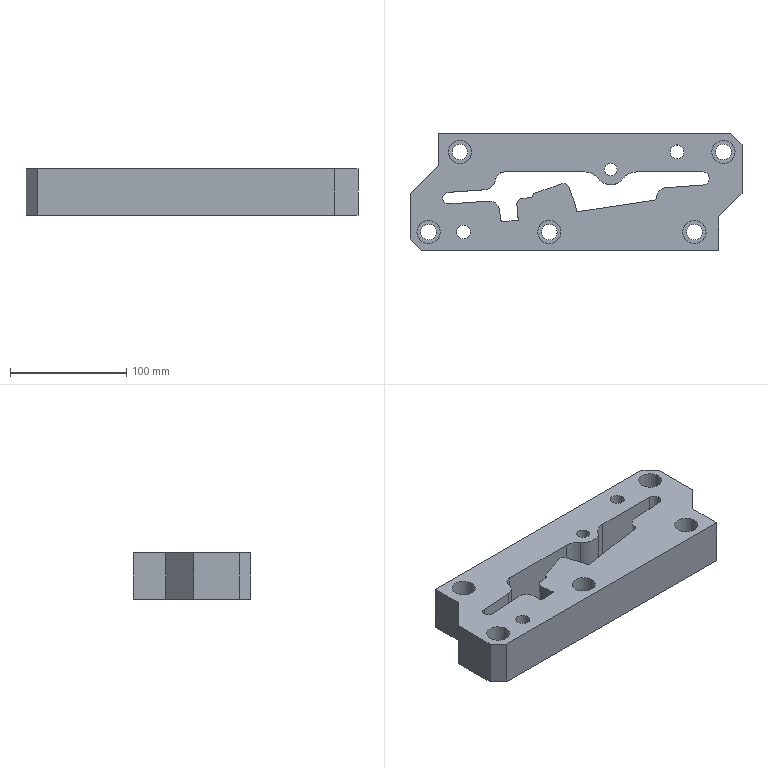Part | NX | features 23 2 | 1 solid | 72 faces | box 286 x 101 x 40 mm | volume 845524 mm3 | plane 38 | cylinder 34 | commonest cylinder face diameters 2 x6 20 x6 13.5 x5 4 x2 10 x2 12.001 x2